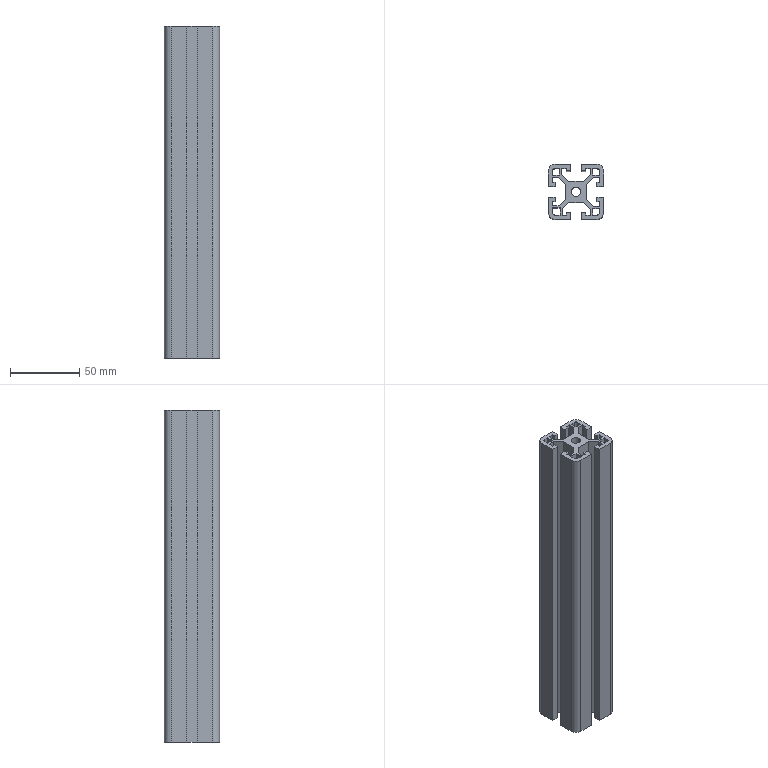Part | STEP file | 4040-240 | 1 solid | 88 faces | box 40 x 40 x 240 mm | volume 168947 mm3 | plane 78 | cylinder 10 | commonest cylinder face diameters 4 x4 10 x4 6.8 x2